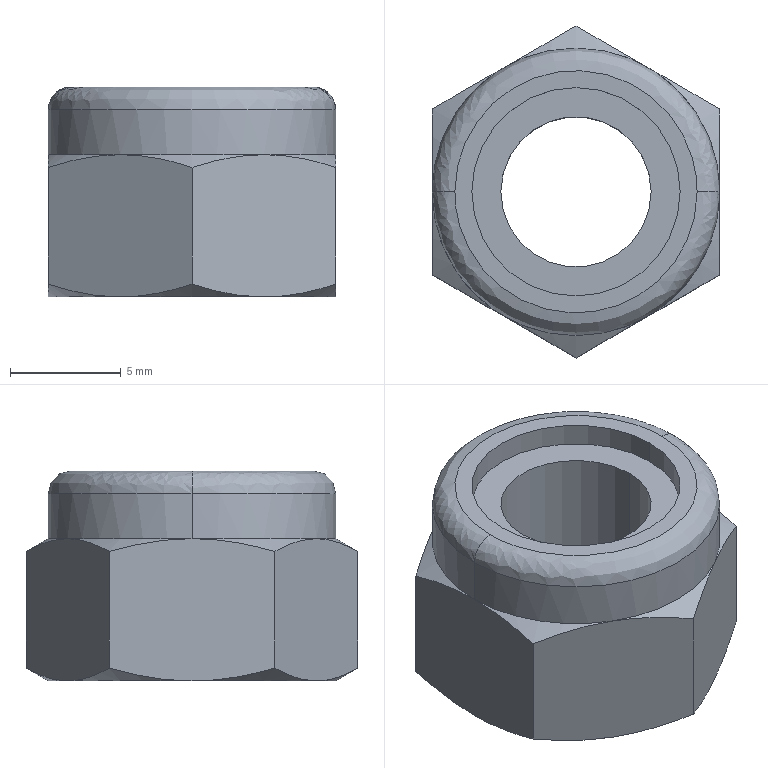Part | STEP file | Flat conveyor mechanism-prevailing torque nut style 1 insert_din_DIN EN ISO 7040 - M8 - N_Default | 1 solid | 33 faces | box 13 x 15.011 x 9.5 mm | volume 952.721 mm3 | cone 14 | plane 9 | cylinder 8 | spline 2 | commonest cylinder face diameters 6.8 x2 8 x2 9.429 x2 13 x2
STEP:
#1=CARTESIAN_POINT('',(5.48,0.,3.06));
#2=VERTEX_POINT('',#1);
#3=CARTESIAN_POINT('',(-5.48,0.,3.06));
#4=VERTEX_POINT('',#3);
#5=CARTESIAN_POINT('',(5.48,0.,3.06));
#6=CARTESIAN_POINT('',(5.48,-10.96,3.06));
#7=CARTESIAN_POINT('',(-5.48,-10.96,3.06));
#8=CARTESIAN_POINT('',(-5.48,0.,3.06));
#9=(BOUNDED_CURVE()B_SPLINE_CURVE(3,(#5,#6,#7,#8),.UNSPECIFIED.,.F.,.F.)B_SPLINE_CURVE_WITH_KNOTS((4,4),(0.,1.),.UNSPECIFIED.)CURVE()GEOMETRIC_REPRESENTATION_ITEM()RATIONAL_B_SPLINE_CURVE((1.,0.3333,0.3333,1.))REPRESENTATION_ITEM(''));
#10=EDGE_CURVE('',#2,#4,#9,.T.);
#11=ORIENTED_EDGE('',*,*,#10,.T.);
#12=CARTESIAN_POINT('',(-6.5,0.,2.04));
#13=VERTEX_POINT('',#12);
#14=CARTESIAN_POINT('',(-5.48,0.,2.04));
#15=DIRECTION('',(0.,-1.,0.));
#16=DIRECTION('',(-1.,0.,0.));
#17=AXIS2_PLACEMENT_3D('',#14,#15,#16);
#18=CIRCLE('',#17,1.02);
#19=EDGE_CURVE('',#4,#13,#18,.T.);
#20=ORIENTED_EDGE('',*,*,#19,.T.);
#21=CARTESIAN_POINT('',(6.5,0.,2.04));
#22=VERTEX_POINT('',#21);
#23=CARTESIAN_POINT('',(0.,0.,2.04));
#24=DIRECTION('',(0.,0.,1.));
#25=DIRECTION('',(1.,0.,0.));
#26=AXIS2_PLACEMENT_3D('',#23,#24,#25);
#27=CIRCLE('',#26,6.5);
#28=EDGE_CURVE('',#13,#22,#27,.T.);
#29=ORIENTED_EDGE('',*,*,#28,.T.);
#30=CARTESIAN_POINT('',(5.48,0.,2.04));
#31=DIRECTION('',(0.,1.,0.));
#32=DIRECTION('',(1.,0.,0.));
#33=AXIS2_PLACEMENT_3D('',#30,#31,#32);
#34=CIRCLE('',#33,1.02);
#35=EDGE_CURVE('',#2,#22,#34,.T.);
#36=ORIENTED_EDGE('',*,*,#35,.F.);
#37=EDGE_LOOP('',(#11,#20,#29,#36));
#38=FACE_OUTER_BOUND('',#37,.T.);
#39=CARTESIAN_POINT('',(-5.48,0.,3.06));
#40=CARTESIAN_POINT('',(-5.48,-10.96,3.06));
#41=CARTESIAN_POINT('',(5.48,-10.96,3.06));
#42=CARTESIAN_POINT('',(5.48,0.,3.06));
#43=CARTESIAN_POINT('',(-6.078,0.,3.06));
#44=CARTESIAN_POINT('',(-6.078,-12.155,3.06));
#45=CARTESIAN_POINT('',(6.078,-12.155,3.06));
#46=CARTESIAN_POINT('',(6.078,0.,3.06));
#47=CARTESIAN_POINT('',(-6.5,0.,2.638));
#48=CARTESIAN_POINT('',(-6.5,-13.,2.638));
#49=CARTESIAN_POINT('',(6.5,-13.,2.638));
#50=CARTESIAN_POINT('',(6.5,0.,2.638));
#51=CARTESIAN_POINT('',(-6.5,0.,2.04));
#52=CARTESIAN_POINT('',(-6.5,-13.,2.04));
#53=CARTESIAN_POINT('',(6.5,-13.,2.04));
#54=CARTESIAN_POINT('',(6.5,0.,2.04));
#55=(BOUNDED_SURFACE()B_SPLINE_SURFACE(3,3,((#39,#40,#41,#42),(#43,#44,#45,#46),(#47,#48,#49,#50),(#51,#52,#53,#54)),.UNSPECIFIED.,.F.,.F.,.T.)B_SPLINE_SURFACE_WITH_KNOTS((4,4),(4,4),(0.,1.),(0.,1.),.UNSPECIFIED.)GEOMETRIC_REPRESENTATION_ITEM()RATIONAL_B_SPLINE_SURFACE(((1.,0.3333,0.3333,1.),(0.8047,0.2682,0.2682,0.8047),(0.8047,0.2682,0.2682,0.8047),(1.,0.3333,0.3333,1.)))REPRESENTATION_ITEM('')SURFACE());
#56=ADVANCED_FACE('',(#38),#55,.T.);
#57=CARTESIAN_POINT('',(-3.4,0.,-5.994));
#58=VERTEX_POINT('',#57);
#59=CARTESIAN_POINT('',(3.4,0.,-5.994));
#60=VERTEX_POINT('',#59);
#61=CARTESIAN_POINT('',(0.,0.,-5.994));
#62=DIRECTION('',(0.,0.,1.));
#63=DIRECTION('',(1.,0.,0.));
#64=AXIS2_PLACEMENT_3D('',#61,#62,#63);
#65=CIRCLE('',#64,3.4);
#66=EDGE_CURVE('',#58,#60,#65,.T.);
#67=ORIENTED_EDGE('',*,*,#66,.F.);
#68=CARTESIAN_POINT('',(-3.4,0.,2.04));
#69=VERTEX_POINT('',#68);
#70=CARTESIAN_POINT('',(-3.4,0.,-6.44));
#71=DIRECTION('',(0.,0.,1.));
#72=VECTOR('',#71,1000.);
#73=LINE('',#70,#72);
#74=EDGE_CURVE('',#58,#69,#73,.T.);
#75=ORIENTED_EDGE('',*,*,#74,.T.);
#76=CARTESIAN_POINT('',(3.4,0.,2.04));
#77=VERTEX_POINT('',#76);
#78=CARTESIAN_POINT('',(0.,0.,2.04));
#79=DIRECTION('',(0.,0.,-1.));
#80=DIRECTION('',(1.,0.,0.));
#81=AXIS2_PLACEMENT_3D('',#78,#79,#80);
#82=CIRCLE('',#81,3.4);
#83=EDGE_CURVE('',#77,#69,#82,.T.);
#84=ORIENTED_EDGE('',*,*,#83,.F.);
#85=CARTESIAN_POINT('',(3.4,0.,-6.44));
#86=DIRECTION('',(0.,0.,1.));
#87=VECTOR('',#86,1000.);
#88=LINE('',#85,#87);
#89=EDGE_CURVE('',#60,#77,#88,.T.);
#90=ORIENTED_EDGE('',*,*,#89,.F.);
#91=EDGE_LOOP('',(#67,#75,#84,#90));
#92=FACE_OUTER_BOUND('',#91,.T.);
#93=CARTESIAN_POINT('',(0.,0.,-6.44));
#94=DIRECTION('',(0.,0.,1.));
#95=DIRECTION('',(1.,0.,0.));
#96=AXIS2_PLACEMENT_3D('',#93,#94,#95);
#97=CYLINDRICAL_SURFACE('',#96,3.4);
#98=ADVANCED_FACE('',(#92),#97,.F.);
#99=ORIENTED_EDGE('',*,*,#66,.T.);
#100=CARTESIAN_POINT('',(4.,0.,-6.415));
#101=VERTEX_POINT('',#100);
#102=CARTESIAN_POINT('',(4.,0.,-6.415));
#103=DIRECTION('',(0.8192,0.,-0.5736));
#104=VECTOR('',#103,1000.);
#105=LINE('',#102,#104);
#106=EDGE_CURVE('',#60,#101,#105,.T.);
#107=ORIENTED_EDGE('',*,*,#106,.T.);
#108=CARTESIAN_POINT('',(-4.,0.,-6.415));
#109=VERTEX_POINT('',#108);
#110=CARTESIAN_POINT('',(0.,0.,-6.415));
#111=DIRECTION('',(0.,0.,1.));
#112=DIRECTION('',(-1.,0.,0.));
#113=AXIS2_PLACEMENT_3D('',#110,#111,#112);
#114=CIRCLE('',#113,4.);
#115=EDGE_CURVE('',#109,#101,#114,.T.);
#116=ORIENTED_EDGE('',*,*,#115,.F.);
#117=CARTESIAN_POINT('',(-4.,0.,-6.415));
#118=DIRECTION('',(-0.8192,0.,-0.5736));
#119=VECTOR('',#118,1000.);
#120=LINE('',#117,#119);
#121=EDGE_CURVE('',#58,#109,#120,.T.);
#122=ORIENTED_EDGE('',*,*,#121,.F.);
#123=EDGE_LOOP('',(#99,#107,#116,#122));
#124=FACE_OUTER_BOUND('',#123,.T.);
#125=CARTESIAN_POINT('',(0.,0.,-6.415));
#126=DIRECTION('',(0.,0.,-1.));
#127=DIRECTION('',(-1.,0.,0.));
#128=AXIS2_PLACEMENT_3D('',#125,#126,#127);
#129=CONICAL_SURFACE('',#128,4.,0.9599);
#130=ADVANCED_FACE('',(#124),#129,.F.);
#131=CARTESIAN_POINT('',(-4.,0.,-6.44));
#132=VERTEX_POINT('',#131);
#133=CARTESIAN_POINT('',(4.,0.,-6.44));
#134=VERTEX_POINT('',#133);
#135=CARTESIAN_POINT('',(0.,0.,-6.44));
#136=DIRECTION('',(0.,0.,1.));
#137=DIRECTION('',(1.,0.,0.));
#138=AXIS2_PLACEMENT_3D('',#135,#136,#137);
#139=CIRCLE('',#138,4.);
#140=EDGE_CURVE('',#132,#134,#139,.T.);
#141=ORIENTED_EDGE('',*,*,#140,.F.);
#142=CARTESIAN_POINT('',(-4.,0.,-25.038));
#143=DIRECTION('',(0.,0.,1.));
#144=VECTOR('',#143,1000.);
#145=LINE('',#142,#144);
#146=EDGE_CURVE('',#132,#109,#145,.T.);
#147=ORIENTED_EDGE('',*,*,#146,.T.);
#148=ORIENTED_EDGE('',*,*,#115,.T.);
#149=CARTESIAN_POINT('',(4.,0.,-25.038));
#150=DIRECTION('',(0.,0.,1.));
#151=VECTOR('',#150,1000.);
#152=LINE('',#149,#151);
#153=EDGE_CURVE('',#134,#101,#152,.T.);
#154=ORIENTED_EDGE('',*,*,#153,.F.);
#155=EDGE_LOOP('',(#141,#147,#148,#154));
#156=FACE_OUTER_BOUND('',#155,.T.);
#157=CARTESIAN_POINT('',(0.,0.,-25.038));
#158=DIRECTION('',(0.,0.,1.));
#159=DIRECTION('',(1.,0.,0.));
#160=AXIS2_PLACEMENT_3D('',#157,#158,#159);
#161=CYLINDRICAL_SURFACE('',#160,4.);
#162=ADVANCED_FACE('',(#156),#161,.F.);
#163=CARTESIAN_POINT('',(4.714,0.,2.04));
#164=VERTEX_POINT('',#163);
#165=CARTESIAN_POINT('',(-4.714,0.,2.04));
#166=VERTEX_POINT('',#165);
#167=CARTESIAN_POINT('',(0.,0.,2.04));
#168=DIRECTION('',(0.,0.,-1.));
#169=DIRECTION('',(1.,0.,0.));
#170=AXIS2_PLACEMENT_3D('',#167,#168,#169);
#171=CIRCLE('',#170,4.714);
#172=EDGE_CURVE('',#164,#166,#171,.T.);
#173=ORIENTED_EDGE('',*,*,#172,.T.);
#174=CARTESIAN_POINT('',(-4.714,0.,3.06));
#175=VERTEX_POINT('',#174);
#176=CARTESIAN_POINT('',(-4.714,0.,9.481));
#177=DIRECTION('',(0.,0.,1.));
#178=VECTOR('',#177,1000.);
#179=LINE('',#176,#178);
#180=EDGE_CURVE('',#166,#175,#179,.T.);
#181=ORIENTED_EDGE('',*,*,#180,.T.);
#182=CARTESIAN_POINT('',(4.714,0.,3.06));
#183=VERTEX_POINT('',#182);
#184=CARTESIAN_POINT('',(0.,0.,3.06));
#185=DIRECTION('',(0.,0.,-1.));
#186=DIRECTION('',(1.,0.,0.));
#187=AXIS2_PLACEMENT_3D('',#184,#185,#186);
#188=CIRCLE('',#187,4.714);
#189=EDGE_CURVE('',#183,#175,#188,.T.);
#190=ORIENTED_EDGE('',*,*,#189,.F.);
#191=CARTESIAN_POINT('',(4.714,0.,9.481));
#192=DIRECTION('',(0.,0.,1.));
#193=VECTOR('',#192,1000.);
#194=LINE('',#191,#193);
#195=EDGE_CURVE('',#164,#183,#194,.T.);
#196=ORIENTED_EDGE('',*,*,#195,.F.);
#197=EDGE_LOOP('',(#173,#181,#190,#196));
#198=FACE_OUTER_BOUND('',#197,.T.);
#199=CARTESIAN_POINT('',(0.,0.,9.481));
#200=DIRECTION('',(0.,0.,1.));
#201=DIRECTION('',(1.,0.,0.));
#202=AXIS2_PLACEMENT_3D('',#199,#200,#201);
#203=CYLINDRICAL_SURFACE('',#202,4.714);
#204=ADVANCED_FACE('',(#198),#203,.F.);
#205=CARTESIAN_POINT('',(-3.25,5.629,0.));
#206=VERTEX_POINT('',#205);
#207=CARTESIAN_POINT('',(-6.5,0.,0.));
#208=VERTEX_POINT('',#207);
#209=CARTESIAN_POINT('',(0.,0.,0.));
#210=DIRECTION('',(0.,0.,1.));
#211=DIRECTION('',(1.,0.,0.));
#212=AXIS2_PLACEMENT_3D('',#209,#210,#211);
#213=CIRCLE('',#212,6.5);
#214=EDGE_CURVE('',#206,#208,#213,.T.);
#215=ORIENTED_EDGE('',*,*,#214,.T.);
#216=CARTESIAN_POINT('',(-6.5,0.,9.481));
#217=DIRECTION('',(0.,0.,1.));
#218=VECTOR('',#217,1000.);
#219=LINE('',#216,#218);
#220=EDGE_CURVE('',#208,#13,#219,.T.);
#221=ORIENTED_EDGE('',*,*,#220,.T.);
#222=CARTESIAN_POINT('',(0.,0.,2.04));
#223=DIRECTION('',(0.,0.,1.));
#224=DIRECTION('',(1.,0.,0.));
#225=AXIS2_PLACEMENT_3D('',#222,#223,#224);
#226=CIRCLE('',#225,6.5);
#227=EDGE_CURVE('',#22,#13,#226,.T.);
#228=ORIENTED_EDGE('',*,*,#227,.F.);
#229=CARTESIAN_POINT('',(6.5,0.,0.));
#230=VERTEX_POINT('',#229);
#231=CARTESIAN_POINT('',(6.5,0.,9.481));
#232=DIRECTION('',(0.,0.,1.));
#233=VECTOR('',#232,1000.);
#234=LINE('',#231,#233);
#235=EDGE_CURVE('',#230,#22,#234,.T.);
#236=ORIENTED_EDGE('',*,*,#235,.F.);
#237=CARTESIAN_POINT('',(3.25,5.629,0.));
#238=VERTEX_POINT('',#237);
#239=CARTESIAN_POINT('',(0.,0.,0.));
#240=DIRECTION('',(0.,0.,1.));
#241=DIRECTION('',(1.,0.,0.));
#242=AXIS2_PLACEMENT_3D('',#239,#240,#241);
#243=CIRCLE('',#242,6.5);
#244=EDGE_CURVE('',#230,#238,#243,.T.);
#245=ORIENTED_EDGE('',*,*,#244,.T.);
#246=CARTESIAN_POINT('',(0.,0.,0.));
#247=DIRECTION('',(0.,0.,1.));
#248=DIRECTION('',(1.,0.,0.));
#249=AXIS2_PLACEMENT_3D('',#246,#247,#248);
#250=CIRCLE('',#249,6.5);
#251=EDGE_CURVE('',#238,#206,#250,.T.);
#252=ORIENTED_EDGE('',*,*,#251,.T.);
#253=EDGE_LOOP('',(#215,#221,#228,#236,#245,#252));
#254=FACE_OUTER_BOUND('',#253,.T.);
#255=CARTESIAN_POINT('',(0.,0.,9.481));
#256=DIRECTION('',(0.,0.,1.));
#257=DIRECTION('',(1.,0.,0.));
#258=AXIS2_PLACEMENT_3D('',#255,#256,#257);
#259=CYLINDRICAL_SURFACE('',#258,6.5);
#260=ADVANCED_FACE('',(#254),#259,.T.);
#261=ORIENTED_EDGE('',*,*,#74,.F.);
#262=CARTESIAN_POINT('',(0.,0.,-5.994));
#263=DIRECTION('',(0.,0.,1.));
#264=DIRECTION('',(1.,0.,0.));
#265=AXIS2_PLACEMENT_3D('',#262,#263,#264);
#266=CIRCLE('',#265,3.4);
#267=EDGE_CURVE('',#60,#58,#266,.T.);
#268=ORIENTED_EDGE('',*,*,#267,.F.);
#269=ORIENTED_EDGE('',*,*,#89,.T.);
#270=CARTESIAN_POINT('',(0.,0.,2.04));
#271=DIRECTION('',(0.,0.,-1.));
#272=DIRECTION('',(1.,0.,0.));
#273=AXIS2_PLACEMENT_3D('',#270,#271,#272);
#274=CIRCLE('',#273,3.4);
#275=EDGE_CURVE('',#69,#77,#274,.T.);
#276=ORIENTED_EDGE('',*,*,#275,.F.);
#277=EDGE_LOOP('',(#261,#268,#269,#276));
#278=FACE_OUTER_BOUND('',#277,.T.);
#279=CARTESIAN_POINT('',(0.,0.,-6.44));
#280=DIRECTION('',(0.,0.,1.));
#281=DIRECTION('',(1.,0.,0.));
#282=AXIS2_PLACEMENT_3D('',#279,#280,#281);
#283=CYLINDRICAL_SURFACE('',#282,3.4);
#284=ADVANCED_FACE('',(#278),#283,.F.);
#285=ORIENTED_EDGE('',*,*,#106,.F.);
#286=ORIENTED_EDGE('',*,*,#267,.T.);
#287=ORIENTED_EDGE('',*,*,#121,.T.);
#288=CARTESIAN_POINT('',(0.,0.,-6.415));
#289=DIRECTION('',(0.,0.,1.));
#290=DIRECTION('',(-1.,0.,0.));
#291=AXIS2_PLACEMENT_3D('',#288,#289,#290);
#292=CIRCLE('',#291,4.);
#293=EDGE_CURVE('',#101,#109,#292,.T.);
#294=ORIENTED_EDGE('',*,*,#293,.F.);
#295=EDGE_LOOP('',(#285,#286,#287,#294));
#296=FACE_OUTER_BOUND('',#295,.T.);
#297=CARTESIAN_POINT('',(0.,0.,-6.415));
#298=DIRECTION('',(0.,0.,-1.));
#299=DIRECTION('',(-1.,0.,0.));
#300=AXIS2_PLACEMENT_3D('',#297,#298,#299);
#301=CONICAL_SURFACE('',#300,4.,0.9599);
#302=ADVANCED_FACE('',(#296),#301,.F.);
#303=ORIENTED_EDGE('',*,*,#172,.F.);
#304=CARTESIAN_POINT('',(0.,0.,2.04));
#305=DIRECTION('',(0.,0.,-1.));
#306=DIRECTION('',(1.,0.,0.));
#307=AXIS2_PLACEMENT_3D('',#304,#305,#306);
#308=CIRCLE('',#307,4.714);
#309=EDGE_CURVE('',#166,#164,#308,.T.);
#310=ORIENTED_EDGE('',*,*,#309,.F.);
#311=EDGE_LOOP('',(#303,#310));
#312=FACE_OUTER_BOUND('',#311,.T.);
#313=ORIENTED_EDGE('',*,*,#83,.T.);
#314=ORIENTED_EDGE('',*,*,#275,.T.);
#315=EDGE_LOOP('',(#313,#314));
#316=FACE_BOUND('',#315,.T.);
#317=CARTESIAN_POINT('',(0.,3.4,2.04));
#318=DIRECTION('',(0.,0.,-1.));
#319=DIRECTION('',(-1.,0.,0.));
#320=AXIS2_PLACEMENT_3D('',#317,#318,#319);
#321=PLANE('',#320);
#322=ADVANCED_FACE('',(#312,#316),#321,.F.);
#323=ORIENTED_EDGE('',*,*,#146,.F.);
#324=CARTESIAN_POINT('',(0.,0.,-6.44));
#325=DIRECTION('',(0.,0.,1.));
#326=DIRECTION('',(1.,0.,0.));
#327=AXIS2_PLACEMENT_3D('',#324,#325,#326);
#328=CIRCLE('',#327,4.);
#329=EDGE_CURVE('',#134,#132,#328,.T.);
#330=ORIENTED_EDGE('',*,*,#329,.F.);
#331=ORIENTED_EDGE('',*,*,#153,.T.);
#332=ORIENTED_EDGE('',*,*,#293,.T.);
#333=EDGE_LOOP('',(#323,#330,#331,#332));
#334=FACE_OUTER_BOUND('',#333,.T.);
#335=CARTESIAN_POINT('',(0.,0.,-25.038));
#336=DIRECTION('',(0.,0.,1.));
#337=DIRECTION('',(1.,0.,0.));
#338=AXIS2_PLACEMENT_3D('',#335,#336,#337);
#339=CYLINDRICAL_SURFACE('',#338,4.);
#340=ADVANCED_FACE('',(#334),#339,.F.);
#341=ORIENTED_EDGE('',*,*,#180,.F.);
#342=ORIENTED_EDGE('',*,*,#309,.T.);
#343=ORIENTED_EDGE('',*,*,#195,.T.);
#344=CARTESIAN_POINT('',(0.,0.,3.06));
#345=DIRECTION('',(0.,0.,-1.));
#346=DIRECTION('',(1.,0.,0.));
#347=AXIS2_PLACEMENT_3D('',#344,#345,#346);
#348=CIRCLE('',#347,4.714);
#349=EDGE_CURVE('',#175,#183,#348,.T.);
#350=ORIENTED_EDGE('',*,*,#349,.F.);
#351=EDGE_LOOP('',(#341,#342,#343,#350));
#352=FACE_OUTER_BOUND('',#351,.T.);
#353=CARTESIAN_POINT('',(0.,0.,9.481));
#354=DIRECTION('',(0.,0.,1.));
#355=DIRECTION('',(1.,0.,0.));
#356=AXIS2_PLACEMENT_3D('',#353,#354,#355);
#357=CYLINDRICAL_SURFACE('',#356,4.714);
#358=ADVANCED_FACE('',(#352),#357,.F.);
#359=CARTESIAN_POINT('',(3.25,-5.629,-6.44));
#360=VERTEX_POINT('',#359);
#361=CARTESIAN_POINT('',(6.5,0.,-6.44));
#362=VERTEX_POINT('',#361);
#363=CARTESIAN_POINT('',(0.,0.,-6.44));
#364=DIRECTION('',(0.,0.,1.));
#365=DIRECTION('',(1.,0.,0.));
#366=AXIS2_PLACEMENT_3D('',#363,#364,#365);
#367=CIRCLE('',#366,6.5);
#368=EDGE_CURVE('',#360,#362,#367,.T.);
#369=ORIENTED_EDGE('',*,*,#368,.F.);
#370=CARTESIAN_POINT('',(-3.25,-5.629,-6.44));
#371=VERTEX_POINT('',#370);
#372=CARTESIAN_POINT('',(0.,0.,-6.44));
#373=DIRECTION('',(0.,0.,1.));
#374=DIRECTION('',(1.,0.,0.));
#375=AXIS2_PLACEMENT_3D('',#372,#373,#374);
#376=CIRCLE('',#375,6.5);
#377=EDGE_CURVE('',#371,#360,#376,.T.);
#378=ORIENTED_EDGE('',*,*,#377,.F.);
#379=CARTESIAN_POINT('',(-6.5,0.,-6.44));
#380=VERTEX_POINT('',#379);
#381=CARTESIAN_POINT('',(0.,0.,-6.44));
#382=DIRECTION('',(0.,0.,1.));
#383=DIRECTION('',(1.,0.,0.));
#384=AXIS2_PLACEMENT_3D('',#381,#382,#383);
#385=CIRCLE('',#384,6.5);
#386=EDGE_CURVE('',#380,#371,#385,.T.);
#387=ORIENTED_EDGE('',*,*,#386,.F.);
#388=CARTESIAN_POINT('',(-3.25,5.629,-6.44));
#389=VERTEX_POINT('',#388);
#390=CARTESIAN_POINT('',(0.,0.,-6.44));
#391=DIRECTION('',(0.,0.,1.));
#392=DIRECTION('',(1.,0.,0.));
#393=AXIS2_PLACEMENT_3D('',#390,#391,#392);
#394=CIRCLE('',#393,6.5);
#395=EDGE_CURVE('',#389,#380,#394,.T.);
#396=ORIENTED_EDGE('',*,*,#395,.F.);
#397=CARTESIAN_POINT('',(3.25,5.629,-6.44));
#398=VERTEX_POINT('',#397);
#399=CARTESIAN_POINT('',(0.,0.,-6.44));
#400=DIRECTION('',(0.,0.,1.));
#401=DIRECTION('',(1.,0.,0.));
#402=AXIS2_PLACEMENT_3D('',#399,#400,#401);
#403=CIRCLE('',#402,6.5);
#404=EDGE_CURVE('',#398,#389,#403,.T.);
#405=ORIENTED_EDGE('',*,*,#404,.F.);
#406=CARTESIAN_POINT('',(0.,0.,-6.44));
#407=DIRECTION('',(0.,0.,1.));
#408=DIRECTION('',(1.,0.,0.));
#409=AXIS2_PLACEMENT_3D('',#406,#407,#408);
#410=CIRCLE('',#409,6.5);
#411=EDGE_CURVE('',#362,#398,#410,.T.);
#412=ORIENTED_EDGE('',*,*,#411,.F.);
#413=EDGE_LOOP('',(#369,#378,#387,#396,#405,#412));
#414=FACE_OUTER_BOUND('',#413,.T.);
#415=ORIENTED_EDGE('',*,*,#329,.T.);
#416=ORIENTED_EDGE('',*,*,#140,.T.);
#417=EDGE_LOOP('',(#415,#416));
#418=FACE_BOUND('',#417,.T.);
#419=CARTESIAN_POINT('',(-13.,0.,-6.44));
#420=DIRECTION('',(0.,0.,1.));
#421=DIRECTION('',(1.,0.,0.));
#422=AXIS2_PLACEMENT_3D('',#419,#420,#421);
#423=PLANE('',#422);
#424=ADVANCED_FACE('',(#414,#418),#423,.F.);
#425=ORIENTED_EDGE('',*,*,#10,.F.);
#426=CARTESIAN_POINT('',(-5.48,0.,3.06));
#427=CARTESIAN_POINT('',(-5.48,10.96,3.06));
#428=CARTESIAN_POINT('',(5.48,10.96,3.06));
#429=CARTESIAN_POINT('',(5.48,0.,3.06));
#430=(BOUNDED_CURVE()B_SPLINE_CURVE(3,(#426,#427,#428,#429),.UNSPECIFIED.,.F.,.T.)B_SPLINE_CURVE_WITH_KNOTS((4,4),(0.,1.),.UNSPECIFIED.)CURVE()GEOMETRIC_REPRESENTATION_ITEM()RATIONAL_B_SPLINE_CURVE((1.,0.3333,0.3333,1.))REPRESENTATION_ITEM(''));
#431=EDGE_CURVE('',#4,#2,#430,.T.);
#432=ORIENTED_EDGE('',*,*,#431,.F.);
#433=EDGE_LOOP('',(#425,#432));
#434=FACE_OUTER_BOUND('',#433,.T.);
#435=ORIENTED_EDGE('',*,*,#189,.T.);
#436=ORIENTED_EDGE('',*,*,#349,.T.);
#437=EDGE_LOOP('',(#435,#436));
#438=FACE_BOUND('',#437,.T.);
#439=CARTESIAN_POINT('',(0.,4.714,3.06));
#440=DIRECTION('',(0.,0.,-1.));
#441=DIRECTION('',(-1.,0.,0.));
#442=AXIS2_PLACEMENT_3D('',#439,#440,#441);
#443=PLANE('',#442);
#444=ADVANCED_FACE('',(#434,#438),#443,.F.);
#445=CARTESIAN_POINT('',(6.5,3.753,-5.859));
#446=VERTEX_POINT('',#445);
#447=CARTESIAN_POINT('',(6.5,3.753,-5.859));
#448=CARTESIAN_POINT('',(6.5,2.527,-6.213));
#449=CARTESIAN_POINT('',(6.5,1.281,-6.44));
#450=CARTESIAN_POINT('',(6.5,0.,-6.44));
#451=B_SPLINE_CURVE_WITH_KNOTS('',3,(#447,#448,#449,#450),.UNSPECIFIED.,.F.,.F.,(4,4),(0.,0.003797),.UNSPECIFIED.);
#452=EDGE_CURVE('',#446,#362,#451,.T.);
#453=ORIENTED_EDGE('',*,*,#452,.T.);
#454=ORIENTED_EDGE('',*,*,#411,.T.);
#455=CARTESIAN_POINT('',(3.25,5.629,-6.44));
#456=CARTESIAN_POINT('',(4.359,4.989,-6.44));
#457=CARTESIAN_POINT('',(5.438,4.366,-6.213));
#458=CARTESIAN_POINT('',(6.5,3.753,-5.859));
#459=B_SPLINE_CURVE_WITH_KNOTS('',3,(#455,#456,#457,#458),.UNSPECIFIED.,.F.,.F.,(4,4),(0.,0.003797),.UNSPECIFIED.);
#460=EDGE_CURVE('',#398,#446,#459,.T.);
#461=ORIENTED_EDGE('',*,*,#460,.T.);
#462=EDGE_LOOP('',(#453,#454,#461));
#463=FACE_OUTER_BOUND('',#462,.T.);
#464=CARTESIAN_POINT('',(0.,0.,-5.856));
#465=DIRECTION('',(0.,0.,1.));
#466=DIRECTION('',(1.,0.,0.));
#467=AXIS2_PLACEMENT_3D('',#464,#465,#466);
#468=CONICAL_SURFACE('',#467,7.512,1.047);
#469=ADVANCED_FACE('',(#463),#468,.T.);
#470=ORIENTED_EDGE('',*,*,#368,.T.);
#471=CARTESIAN_POINT('',(6.5,-3.753,-5.859));
#472=VERTEX_POINT('',#471);
#473=CARTESIAN_POINT('',(6.5,0.,-6.44));
#474=CARTESIAN_POINT('',(6.5,-1.281,-6.44));
#475=CARTESIAN_POINT('',(6.5,-2.527,-6.213));
#476=CARTESIAN_POINT('',(6.5,-3.753,-5.859));
#477=B_SPLINE_CURVE_WITH_KNOTS('',3,(#473,#474,#475,#476),.UNSPECIFIED.,.F.,.F.,(4,4),(0.,0.003797),.UNSPECIFIED.);
#478=EDGE_CURVE('',#362,#472,#477,.T.);
#479=ORIENTED_EDGE('',*,*,#478,.T.);
#480=CARTESIAN_POINT('',(6.5,-3.753,-5.859));
#481=CARTESIAN_POINT('',(5.438,-4.366,-6.213));
#482=CARTESIAN_POINT('',(4.359,-4.989,-6.44));
#483=CARTESIAN_POINT('',(3.25,-5.629,-6.44));
#484=B_SPLINE_CURVE_WITH_KNOTS('',3,(#480,#481,#482,#483),.UNSPECIFIED.,.F.,.F.,(4,4),(0.,0.003797),.UNSPECIFIED.);
#485=EDGE_CURVE('',#472,#360,#484,.T.);
#486=ORIENTED_EDGE('',*,*,#485,.T.);
#487=EDGE_LOOP('',(#470,#479,#486));
#488=FACE_OUTER_BOUND('',#487,.T.);
#489=CARTESIAN_POINT('',(0.,0.,-5.856));
#490=DIRECTION('',(0.,0.,1.));
#491=DIRECTION('',(1.,0.,0.));
#492=AXIS2_PLACEMENT_3D('',#489,#490,#491);
#493=CONICAL_SURFACE('',#492,7.512,1.047);
#494=ADVANCED_FACE('',(#488),#493,.T.);
#495=CARTESIAN_POINT('',(0.000000038,-7.506,-5.859));
#496=VERTEX_POINT('',#495);
#497=CARTESIAN_POINT('',(0.000000038,-7.506,-5.859));
#498=CARTESIAN_POINT('',(-1.062,-6.892,-6.213));
#499=CARTESIAN_POINT('',(-2.141,-6.27,-6.44));
#500=CARTESIAN_POINT('',(-3.25,-5.629,-6.44));
#501=B_SPLINE_CURVE_WITH_KNOTS('',3,(#497,#498,#499,#500),.UNSPECIFIED.,.F.,.F.,(4,4),(0.,0.003797),.UNSPECIFIED.);
#502=EDGE_CURVE('',#496,#371,#501,.T.);
#503=ORIENTED_EDGE('',*,*,#502,.T.);
#504=ORIENTED_EDGE('',*,*,#377,.T.);
#505=CARTESIAN_POINT('',(3.25,-5.629,-6.44));
#506=CARTESIAN_POINT('',(2.141,-6.27,-6.44));
#507=CARTESIAN_POINT('',(1.062,-6.892,-6.213));
#508=CARTESIAN_POINT('',(0.000000038,-7.506,-5.859));
#509=B_SPLINE_CURVE_WITH_KNOTS('',3,(#505,#506,#507,#508),.UNSPECIFIED.,.F.,.F.,(4,4),(0.,0.003797),.UNSPECIFIED.);
#510=EDGE_CURVE('',#360,#496,#509,.T.);
#511=ORIENTED_EDGE('',*,*,#510,.T.);
#512=EDGE_LOOP('',(#503,#504,#511));
#513=FACE_OUTER_BOUND('',#512,.T.);
#514=CARTESIAN_POINT('',(0.,0.,-5.856));
#515=DIRECTION('',(0.,0.,1.));
#516=DIRECTION('',(1.,0.,0.));
#517=AXIS2_PLACEMENT_3D('',#514,#515,#516);
#518=CONICAL_SURFACE('',#517,7.512,1.047);
#519=ADVANCED_FACE('',(#513),#518,.T.);
#520=CARTESIAN_POINT('',(-6.5,-3.753,-5.859));
#521=VERTEX_POINT('',#520);
#522=CARTESIAN_POINT('',(-6.5,-3.753,-5.859));
#523=CARTESIAN_POINT('',(-6.5,-2.527,-6.213));
#524=CARTESIAN_POINT('',(-6.5,-1.281,-6.44));
#525=CARTESIAN_POINT('',(-6.5,0.,-6.44));
#526=B_SPLINE_CURVE_WITH_KNOTS('',3,(#522,#523,#524,#525),.UNSPECIFIED.,.F.,.F.,(4,4),(0.,0.003797),.UNSPECIFIED.);
#527=EDGE_CURVE('',#521,#380,#526,.T.);
#528=ORIENTED_EDGE('',*,*,#527,.T.);
#529=ORIENTED_EDGE('',*,*,#386,.T.);
#530=CARTESIAN_POINT('',(-3.25,-5.629,-6.44));
#531=CARTESIAN_POINT('',(-4.359,-4.989,-6.44));
#532=CARTESIAN_POINT('',(-5.438,-4.366,-6.213));
#533=CARTESIAN_POINT('',(-6.5,-3.753,-5.859));
#534=B_SPLINE_CURVE_WITH_KNOTS('',3,(#530,#531,#532,#533),.UNSPECIFIED.,.F.,.F.,(4,4),(0.,0.003797),.UNSPECIFIED.);
#535=EDGE_CURVE('',#371,#521,#534,.T.);
#536=ORIENTED_EDGE('',*,*,#535,.T.);
#537=EDGE_LOOP('',(#528,#529,#536));
#538=FACE_OUTER_BOUND('',#537,.T.);
#539=CARTESIAN_POINT('',(0.,0.,-5.856));
#540=DIRECTION('',(0.,0.,1.));
#541=DIRECTION('',(1.,0.,0.));
#542=AXIS2_PLACEMENT_3D('',#539,#540,#541);
#543=CONICAL_SURFACE('',#542,7.512,1.047);
#544=ADVANCED_FACE('',(#538),#543,.T.);
#545=ORIENTED_EDGE('',*,*,#395,.T.);
#546=CARTESIAN_POINT('',(-6.5,3.753,-5.859));
#547=VERTEX_POINT('',#546);
#548=CARTESIAN_POINT('',(-6.5,0.,-6.44));
#549=CARTESIAN_POINT('',(-6.5,1.281,-6.44));
#550=CARTESIAN_POINT('',(-6.5,2.527,-6.213));
#551=CARTESIAN_POINT('',(-6.5,3.753,-5.859));
#552=B_SPLINE_CURVE_WITH_KNOTS('',3,(#548,#549,#550,#551),.UNSPECIFIED.,.F.,.F.,(4,4),(0.,0.003797),.UNSPECIFIED.);
#553=EDGE_CURVE('',#380,#547,#552,.T.);
#554=ORIENTED_EDGE('',*,*,#553,.T.);
#555=CARTESIAN_POINT('',(-6.5,3.753,-5.859));
#556=CARTESIAN_POINT('',(-5.438,4.366,-6.213));
#557=CARTESIAN_POINT('',(-4.359,4.989,-6.44));
#558=CARTESIAN_POINT('',(-3.25,5.629,-6.44));
#559=B_SPLINE_CURVE_WITH_KNOTS('',3,(#555,#556,#557,#558),.UNSPECIFIED.,.F.,.F.,(4,4),(0.,0.003797),.UNSPECIFIED.);
#560=EDGE_CURVE('',#547,#389,#559,.T.);
#561=ORIENTED_EDGE('',*,*,#560,.T.);
#562=EDGE_LOOP('',(#545,#554,#561));
#563=FACE_OUTER_BOUND('',#562,.T.);
#564=CARTESIAN_POINT('',(0.,0.,-5.856));
#565=DIRECTION('',(0.,0.,1.));
#566=DIRECTION('',(1.,0.,0.));
#567=AXIS2_PLACEMENT_3D('',#564,#565,#566);
#568=CONICAL_SURFACE('',#567,7.512,1.047);
#569=ADVANCED_FACE('',(#563),#568,.T.);
#570=CARTESIAN_POINT('',(-0.000000038,7.506,-5.859));
#571=VERTEX_POINT('',#570);
#572=CARTESIAN_POINT('',(-0.000000038,7.506,-5.859));
#573=CARTESIAN_POINT('',(1.062,6.892,-6.213));
#574=CARTESIAN_POINT('',(2.141,6.27,-6.44));
#575=CARTESIAN_POINT('',(3.25,5.629,-6.44));
#576=B_SPLINE_CURVE_WITH_KNOTS('',3,(#572,#573,#574,#575),.UNSPECIFIED.,.F.,.F.,(4,4),(0.,0.003797),.UNSPECIFIED.);
#577=EDGE_CURVE('',#571,#398,#576,.T.);
#578=ORIENTED_EDGE('',*,*,#577,.T.);
#579=ORIENTED_EDGE('',*,*,#404,.T.);
#580=CARTESIAN_POINT('',(-3.25,5.629,-6.44));
#581=CARTESIAN_POINT('',(-2.141,6.27,-6.44));
#582=CARTESIAN_POINT('',(-1.062,6.892,-6.213));
#583=CARTESIAN_POINT('',(-0.000000038,7.506,-5.859));
#584=B_SPLINE_CURVE_WITH_KNOTS('',3,(#580,#581,#582,#583),.UNSPECIFIED.,.F.,.F.,(4,4),(0.,0.003797),.UNSPECIFIED.);
#585=EDGE_CURVE('',#389,#571,#584,.T.);
#586=ORIENTED_EDGE('',*,*,#585,.T.);
#587=EDGE_LOOP('',(#578,#579,#586));
#588=FACE_OUTER_BOUND('',#587,.T.);
#589=CARTESIAN_POINT('',(0.,0.,-5.856));
#590=DIRECTION('',(0.,0.,1.));
#591=DIRECTION('',(1.,0.,0.));
#592=AXIS2_PLACEMENT_3D('',#589,#590,#591);
#593=CONICAL_SURFACE('',#592,7.512,1.047);
#594=ADVANCED_FACE('',(#588),#593,.T.);
#595=ORIENTED_EDGE('',*,*,#19,.F.);
#596=ORIENTED_EDGE('',*,*,#431,.T.);
#597=ORIENTED_EDGE('',*,*,#35,.T.);
#598=ORIENTED_EDGE('',*,*,#227,.T.);
#599=EDGE_LOOP('',(#595,#596,#597,#598));
#600=FACE_OUTER_BOUND('',#599,.T.);
#601=CARTESIAN_POINT('',(5.48,0.,3.06));
#602=CARTESIAN_POINT('',(5.48,10.96,3.06));
#603=CARTESIAN_POINT('',(-5.48,10.96,3.06));
#604=CARTESIAN_POINT('',(-5.48,0.,3.06));
#605=CARTESIAN_POINT('',(6.078,0.,3.06));
#606=CARTESIAN_POINT('',(6.078,12.155,3.06));
#607=CARTESIAN_POINT('',(-6.078,12.155,3.06));
#608=CARTESIAN_POINT('',(-6.078,0.,3.06));
#609=CARTESIAN_POINT('',(6.5,0.,2.638));
#610=CARTESIAN_POINT('',(6.5,13.,2.638));
#611=CARTESIAN_POINT('',(-6.5,13.,2.638));
#612=CARTESIAN_POINT('',(-6.5,0.,2.638));
#613=CARTESIAN_POINT('',(6.5,0.,2.04));
#614=CARTESIAN_POINT('',(6.5,13.,2.04));
#615=CARTESIAN_POINT('',(-6.5,13.,2.04));
#616=CARTESIAN_POINT('',(-6.5,0.,2.04));
#617=(BOUNDED_SURFACE()B_SPLINE_SURFACE(3,3,((#601,#602,#603,#604),(#605,#606,#607,#608),(#609,#610,#611,#612),(#613,#614,#615,#616)),.UNSPECIFIED.,.F.,.F.,.T.)B_SPLINE_SURFACE_WITH_KNOTS((4,4),(4,4),(0.,1.),(0.,1.),.UNSPECIFIED.)GEOMETRIC_REPRESENTATION_ITEM()RATIONAL_B_SPLINE_SURFACE(((1.,0.3333,0.3333,1.),(0.8047,0.2682,0.2682,0.8047),(0.8047,0.2682,0.2682,0.8047),(1.,0.3333,0.3333,1.)))REPRESENTATION_ITEM('')SURFACE());
#618=ADVANCED_FACE('',(#600),#617,.T.);
#619=CARTESIAN_POINT('',(6.5,-3.753,-0.5806));
#620=VERTEX_POINT('',#619);
#621=CARTESIAN_POINT('',(6.5,-3.753,-6.44));
#622=DIRECTION('',(0.,0.,1.));
#623=VECTOR('',#622,1000.);
#624=LINE('',#621,#623);
#625=EDGE_CURVE('',#472,#620,#624,.T.);
#626=ORIENTED_EDGE('',*,*,#625,.F.);
#627=ORIENTED_EDGE('',*,*,#478,.F.);
#628=ORIENTED_EDGE('',*,*,#452,.F.);
#629=CARTESIAN_POINT('',(6.5,3.753,-0.5806));
#630=VERTEX_POINT('',#629);
#631=CARTESIAN_POINT('',(6.5,3.753,-6.44));
#632=DIRECTION('',(0.,0.,-1.));
#633=VECTOR('',#632,1000.);
#634=LINE('',#631,#633);
#635=EDGE_CURVE('',#630,#446,#634,.T.);
#636=ORIENTED_EDGE('',*,*,#635,.F.);
#637=CARTESIAN_POINT('',(6.5,0.,0.));
#638=CARTESIAN_POINT('',(6.5,1.281,0.));
#639=CARTESIAN_POINT('',(6.5,2.527,-0.2266));
#640=CARTESIAN_POINT('',(6.5,3.753,-0.5806));
#641=B_SPLINE_CURVE_WITH_KNOTS('',3,(#637,#638,#639,#640),.UNSPECIFIED.,.F.,.F.,(4,4),(0.,0.003797),.UNSPECIFIED.);
#642=EDGE_CURVE('',#230,#630,#641,.T.);
#643=ORIENTED_EDGE('',*,*,#642,.F.);
#644=CARTESIAN_POINT('',(6.5,-3.753,-0.5806));
#645=CARTESIAN_POINT('',(6.5,-2.527,-0.2266));
#646=CARTESIAN_POINT('',(6.5,-1.281,0.));
#647=CARTESIAN_POINT('',(6.5,0.,0.));
#648=B_SPLINE_CURVE_WITH_KNOTS('',3,(#644,#645,#646,#647),.UNSPECIFIED.,.F.,.F.,(4,4),(0.,0.003797),.UNSPECIFIED.);
#649=EDGE_CURVE('',#620,#230,#648,.T.);
#650=ORIENTED_EDGE('',*,*,#649,.F.);
#651=EDGE_LOOP('',(#626,#627,#628,#636,#643,#650));
#652=FACE_OUTER_BOUND('',#651,.T.);
#653=CARTESIAN_POINT('',(6.5,3.753,-6.44));
#654=DIRECTION('',(-1.,0.,0.));
#655=DIRECTION('',(0.,0.,1.));
#656=AXIS2_PLACEMENT_3D('',#653,#654,#655);
#657=PLANE('',#656);
#658=ADVANCED_FACE('',(#652),#657,.F.);
#659=ORIENTED_EDGE('',*,*,#460,.F.);
#660=ORIENTED_EDGE('',*,*,#577,.F.);
#661=CARTESIAN_POINT('',(0.,7.506,-0.5806));
#662=VERTEX_POINT('',#661);
#663=CARTESIAN_POINT('',(0.,7.506,-6.44));
#664=DIRECTION('',(0.,0.,1.));
#665=VECTOR('',#664,1000.);
#666=LINE('',#663,#665);
#667=EDGE_CURVE('',#571,#662,#666,.T.);
#668=ORIENTED_EDGE('',*,*,#667,.T.);
#669=CARTESIAN_POINT('',(0.,7.506,-0.5806));
#670=CARTESIAN_POINT('',(1.062,6.892,-0.2266));
#671=CARTESIAN_POINT('',(2.141,6.27,0.));
#672=CARTESIAN_POINT('',(3.25,5.629,0.));
#673=B_SPLINE_CURVE_WITH_KNOTS('',3,(#669,#670,#671,#672),.UNSPECIFIED.,.F.,.F.,(4,4),(0.,0.003797),.UNSPECIFIED.);
#674=EDGE_CURVE('',#662,#238,#673,.T.);
#675=ORIENTED_EDGE('',*,*,#674,.T.);
#676=CARTESIAN_POINT('',(3.25,5.629,0.));
#677=CARTESIAN_POINT('',(4.359,4.989,0.));
#678=CARTESIAN_POINT('',(5.438,4.366,-0.2266));
#679=CARTESIAN_POINT('',(6.5,3.753,-0.5806));
#680=B_SPLINE_CURVE_WITH_KNOTS('',3,(#676,#677,#678,#679),.UNSPECIFIED.,.F.,.F.,(4,4),(0.,0.003797),.UNSPECIFIED.);
#681=EDGE_CURVE('',#238,#630,#680,.T.);
#682=ORIENTED_EDGE('',*,*,#681,.T.);
#683=ORIENTED_EDGE('',*,*,#635,.T.);
#684=EDGE_LOOP('',(#659,#660,#668,#675,#682,#683));
#685=FACE_OUTER_BOUND('',#684,.T.);
#686=CARTESIAN_POINT('',(6.5,3.753,-6.44));
#687=DIRECTION('',(0.5,0.866,0.));
#688=DIRECTION('',(-0.866,0.5,0.));
#689=AXIS2_PLACEMENT_3D('',#686,#687,#688);
#690=PLANE('',#689);
#691=ADVANCED_FACE('',(#685),#690,.T.);
#692=ORIENTED_EDGE('',*,*,#510,.F.);
#693=ORIENTED_EDGE('',*,*,#485,.F.);
#694=ORIENTED_EDGE('',*,*,#625,.T.);
#695=CARTESIAN_POINT('',(3.25,-5.629,0.));
#696=VERTEX_POINT('',#695);
#697=CARTESIAN_POINT('',(6.5,-3.753,-0.5806));
#698=CARTESIAN_POINT('',(5.438,-4.366,-0.2266));
#699=CARTESIAN_POINT('',(4.359,-4.989,0.));
#700=CARTESIAN_POINT('',(3.25,-5.629,0.));
#701=B_SPLINE_CURVE_WITH_KNOTS('',3,(#697,#698,#699,#700),.UNSPECIFIED.,.F.,.F.,(4,4),(0.,0.003797),.UNSPECIFIED.);
#702=EDGE_CURVE('',#620,#696,#701,.T.);
#703=ORIENTED_EDGE('',*,*,#702,.T.);
#704=CARTESIAN_POINT('',(0.,-7.506,-0.5806));
#705=VERTEX_POINT('',#704);
#706=CARTESIAN_POINT('',(3.25,-5.629,0.));
#707=CARTESIAN_POINT('',(2.141,-6.27,0.));
#708=CARTESIAN_POINT('',(1.062,-6.892,-0.2266));
#709=CARTESIAN_POINT('',(0.,-7.506,-0.5806));
#710=B_SPLINE_CURVE_WITH_KNOTS('',3,(#706,#707,#708,#709),.UNSPECIFIED.,.F.,.F.,(4,4),(0.,0.003797),.UNSPECIFIED.);
#711=EDGE_CURVE('',#696,#705,#710,.T.);
#712=ORIENTED_EDGE('',*,*,#711,.T.);
#713=CARTESIAN_POINT('',(0.,-7.506,-6.44));
#714=DIRECTION('',(0.,0.,-1.));
#715=VECTOR('',#714,1000.);
#716=LINE('',#713,#715);
#717=EDGE_CURVE('',#705,#496,#716,.T.);
#718=ORIENTED_EDGE('',*,*,#717,.T.);
#719=EDGE_LOOP('',(#692,#693,#694,#703,#712,#718));
#720=FACE_OUTER_BOUND('',#719,.T.);
#721=CARTESIAN_POINT('',(0.,-7.506,-6.44));
#722=DIRECTION('',(0.5,-0.866,0.));
#723=DIRECTION('',(0.866,0.5,0.));
#724=AXIS2_PLACEMENT_3D('',#721,#722,#723);
#725=PLANE('',#724);
#726=ADVANCED_FACE('',(#720),#725,.T.);
#727=ORIENTED_EDGE('',*,*,#535,.F.);
#728=ORIENTED_EDGE('',*,*,#502,.F.);
#729=ORIENTED_EDGE('',*,*,#717,.F.);
#730=CARTESIAN_POINT('',(-3.25,-5.629,0.));
#731=VERTEX_POINT('',#730);
#732=CARTESIAN_POINT('',(0.,-7.506,-0.5806));
#733=CARTESIAN_POINT('',(-1.062,-6.892,-0.2266));
#734=CARTESIAN_POINT('',(-2.141,-6.27,0.));
#735=CARTESIAN_POINT('',(-3.25,-5.629,0.));
#736=B_SPLINE_CURVE_WITH_KNOTS('',3,(#732,#733,#734,#735),.UNSPECIFIED.,.F.,.F.,(4,4),(0.,0.003797),.UNSPECIFIED.);
#737=EDGE_CURVE('',#705,#731,#736,.T.);
#738=ORIENTED_EDGE('',*,*,#737,.T.);
#739=CARTESIAN_POINT('',(-6.5,-3.753,-0.5806));
#740=VERTEX_POINT('',#739);
#741=CARTESIAN_POINT('',(-3.25,-5.629,0.));
#742=CARTESIAN_POINT('',(-4.359,-4.989,0.));
#743=CARTESIAN_POINT('',(-5.438,-4.366,-0.2266));
#744=CARTESIAN_POINT('',(-6.5,-3.753,-0.5806));
#745=B_SPLINE_CURVE_WITH_KNOTS('',3,(#741,#742,#743,#744),.UNSPECIFIED.,.F.,.F.,(4,4),(0.,0.003797),.UNSPECIFIED.);
#746=EDGE_CURVE('',#731,#740,#745,.T.);
#747=ORIENTED_EDGE('',*,*,#746,.T.);
#748=CARTESIAN_POINT('',(-6.5,-3.753,-6.44));
#749=DIRECTION('',(0.,0.,-1.));
#750=VECTOR('',#749,1000.);
#751=LINE('',#748,#750);
#752=EDGE_CURVE('',#740,#521,#751,.T.);
#753=ORIENTED_EDGE('',*,*,#752,.T.);
#754=EDGE_LOOP('',(#727,#728,#729,#738,#747,#753));
#755=FACE_OUTER_BOUND('',#754,.T.);
#756=CARTESIAN_POINT('',(-6.5,-3.753,-6.44));
#757=DIRECTION('',(-0.5,-0.866,0.));
#758=DIRECTION('',(0.866,-0.5,0.));
#759=AXIS2_PLACEMENT_3D('',#756,#757,#758);
#760=PLANE('',#759);
#761=ADVANCED_FACE('',(#755),#760,.T.);
#762=ORIENTED_EDGE('',*,*,#553,.F.);
#763=ORIENTED_EDGE('',*,*,#527,.F.);
#764=ORIENTED_EDGE('',*,*,#752,.F.);
#765=CARTESIAN_POINT('',(-6.5,-3.753,-0.5806));
#766=CARTESIAN_POINT('',(-6.5,-2.527,-0.2266));
#767=CARTESIAN_POINT('',(-6.5,-1.281,0.));
#768=CARTESIAN_POINT('',(-6.5,0.,0.));
#769=B_SPLINE_CURVE_WITH_KNOTS('',3,(#765,#766,#767,#768),.UNSPECIFIED.,.F.,.F.,(4,4),(0.,0.003797),.UNSPECIFIED.);
#770=EDGE_CURVE('',#740,#208,#769,.T.);
#771=ORIENTED_EDGE('',*,*,#770,.T.);
#772=CARTESIAN_POINT('',(-6.5,3.753,-0.5806));
#773=VERTEX_POINT('',#772);
#774=CARTESIAN_POINT('',(-6.5,0.,0.));
#775=CARTESIAN_POINT('',(-6.5,1.281,0.));
#776=CARTESIAN_POINT('',(-6.5,2.527,-0.2266));
#777=CARTESIAN_POINT('',(-6.5,3.753,-0.5806));
#778=B_SPLINE_CURVE_WITH_KNOTS('',3,(#774,#775,#776,#777),.UNSPECIFIED.,.F.,.F.,(4,4),(0.,0.003797),.UNSPECIFIED.);
#779=EDGE_CURVE('',#208,#773,#778,.T.);
#780=ORIENTED_EDGE('',*,*,#779,.T.);
#781=CARTESIAN_POINT('',(-6.5,3.753,-6.44));
#782=DIRECTION('',(0.,0.,-1.));
#783=VECTOR('',#782,1000.);
#784=LINE('',#781,#783);
#785=EDGE_CURVE('',#773,#547,#784,.T.);
#786=ORIENTED_EDGE('',*,*,#785,.T.);
#787=EDGE_LOOP('',(#762,#763,#764,#771,#780,#786));
#788=FACE_OUTER_BOUND('',#787,.T.);
#789=CARTESIAN_POINT('',(-6.5,3.753,-6.44));
#790=DIRECTION('',(-1.,0.,0.));
#791=DIRECTION('',(0.,0.,1.));
#792=AXIS2_PLACEMENT_3D('',#789,#790,#791);
#793=PLANE('',#792);
#794=ADVANCED_FACE('',(#788),#793,.T.);
#795=ORIENTED_EDGE('',*,*,#585,.F.);
#796=ORIENTED_EDGE('',*,*,#560,.F.);
#797=ORIENTED_EDGE('',*,*,#785,.F.);
#798=CARTESIAN_POINT('',(-6.5,3.753,-0.5806));
#799=CARTESIAN_POINT('',(-5.438,4.366,-0.2266));
#800=CARTESIAN_POINT('',(-4.359,4.989,0.));
#801=CARTESIAN_POINT('',(-3.25,5.629,0.));
#802=B_SPLINE_CURVE_WITH_KNOTS('',3,(#798,#799,#800,#801),.UNSPECIFIED.,.F.,.F.,(4,4),(0.,0.003797),.UNSPECIFIED.);
#803=EDGE_CURVE('',#773,#206,#802,.T.);
#804=ORIENTED_EDGE('',*,*,#803,.T.);
#805=CARTESIAN_POINT('',(-3.25,5.629,0.));
#806=CARTESIAN_POINT('',(-2.141,6.27,0.));
#807=CARTESIAN_POINT('',(-1.062,6.892,-0.2266));
#808=CARTESIAN_POINT('',(0.,7.506,-0.5806));
#809=B_SPLINE_CURVE_WITH_KNOTS('',3,(#805,#806,#807,#808),.UNSPECIFIED.,.F.,.F.,(4,4),(0.,0.003797),.UNSPECIFIED.);
#810=EDGE_CURVE('',#206,#662,#809,.T.);
#811=ORIENTED_EDGE('',*,*,#810,.T.);
#812=ORIENTED_EDGE('',*,*,#667,.F.);
#813=EDGE_LOOP('',(#795,#796,#797,#804,#811,#812));
#814=FACE_OUTER_BOUND('',#813,.T.);
#815=CARTESIAN_POINT('',(0.,7.506,-6.44));
#816=DIRECTION('',(-0.5,0.866,0.));
#817=DIRECTION('',(-0.866,-0.5,0.));
#818=AXIS2_PLACEMENT_3D('',#815,#816,#817);
#819=PLANE('',#818);
#820=ADVANCED_FACE('',(#814),#819,.T.);
#821=ORIENTED_EDGE('',*,*,#220,.F.);
#822=CARTESIAN_POINT('',(0.,0.,0.));
#823=DIRECTION('',(0.,0.,1.));
#824=DIRECTION('',(1.,0.,0.));
#825=AXIS2_PLACEMENT_3D('',#822,#823,#824);
#826=CIRCLE('',#825,6.5);
#827=EDGE_CURVE('',#208,#731,#826,.T.);
#828=ORIENTED_EDGE('',*,*,#827,.T.);
#829=CARTESIAN_POINT('',(0.,0.,0.));
#830=DIRECTION('',(0.,0.,1.));
#831=DIRECTION('',(1.,0.,0.));
#832=AXIS2_PLACEMENT_3D('',#829,#830,#831);
#833=CIRCLE('',#832,6.5);
#834=EDGE_CURVE('',#731,#696,#833,.T.);
#835=ORIENTED_EDGE('',*,*,#834,.T.);
#836=CARTESIAN_POINT('',(0.,0.,0.));
#837=DIRECTION('',(0.,0.,1.));
#838=DIRECTION('',(1.,0.,0.));
#839=AXIS2_PLACEMENT_3D('',#836,#837,#838);
#840=CIRCLE('',#839,6.5);
#841=EDGE_CURVE('',#696,#230,#840,.T.);
#842=ORIENTED_EDGE('',*,*,#841,.T.);
#843=ORIENTED_EDGE('',*,*,#235,.T.);
#844=ORIENTED_EDGE('',*,*,#28,.F.);
#845=EDGE_LOOP('',(#821,#828,#835,#842,#843,#844));
#846=FACE_OUTER_BOUND('',#845,.T.);
#847=CARTESIAN_POINT('',(0.,0.,9.481));
#848=DIRECTION('',(0.,0.,1.));
#849=DIRECTION('',(1.,0.,0.));
#850=AXIS2_PLACEMENT_3D('',#847,#848,#849);
#851=CYLINDRICAL_SURFACE('',#850,6.5);
#852=ADVANCED_FACE('',(#846),#851,.T.);
#853=ORIENTED_EDGE('',*,*,#841,.F.);
#854=ORIENTED_EDGE('',*,*,#702,.F.);
#855=ORIENTED_EDGE('',*,*,#649,.T.);
#856=EDGE_LOOP('',(#853,#854,#855));
#857=FACE_OUTER_BOUND('',#856,.T.);
#858=CARTESIAN_POINT('',(0.,0.,-0.584));
#859=DIRECTION('',(0.,0.,-1.));
#860=DIRECTION('',(-1.,0.,0.));
#861=AXIS2_PLACEMENT_3D('',#858,#859,#860);
#862=CONICAL_SURFACE('',#861,7.512,1.047);
#863=ADVANCED_FACE('',(#857),#862,.T.);
#864=ORIENTED_EDGE('',*,*,#642,.T.);
#865=ORIENTED_EDGE('',*,*,#681,.F.);
#866=ORIENTED_EDGE('',*,*,#244,.F.);
#867=EDGE_LOOP('',(#864,#865,#866));
#868=FACE_OUTER_BOUND('',#867,.T.);
#869=CARTESIAN_POINT('',(0.,0.,-0.584));
#870=DIRECTION('',(0.,0.,-1.));
#871=DIRECTION('',(-1.,0.,0.));
#872=AXIS2_PLACEMENT_3D('',#869,#870,#871);
#873=CONICAL_SURFACE('',#872,7.512,1.047);
#874=ADVANCED_FACE('',(#868),#873,.T.);
#875=ORIENTED_EDGE('',*,*,#674,.F.);
#876=ORIENTED_EDGE('',*,*,#810,.F.);
#877=ORIENTED_EDGE('',*,*,#251,.F.);
#878=EDGE_LOOP('',(#875,#876,#877));
#879=FACE_OUTER_BOUND('',#878,.T.);
#880=CARTESIAN_POINT('',(0.,0.,-0.584));
#881=DIRECTION('',(0.,0.,-1.));
#882=DIRECTION('',(-1.,0.,0.));
#883=AXIS2_PLACEMENT_3D('',#880,#881,#882);
#884=CONICAL_SURFACE('',#883,7.512,1.047);
#885=ADVANCED_FACE('',(#879),#884,.T.);
#886=ORIENTED_EDGE('',*,*,#737,.F.);
#887=ORIENTED_EDGE('',*,*,#711,.F.);
#888=ORIENTED_EDGE('',*,*,#834,.F.);
#889=EDGE_LOOP('',(#886,#887,#888));
#890=FACE_OUTER_BOUND('',#889,.T.);
#891=CARTESIAN_POINT('',(0.,0.,-0.584));
#892=DIRECTION('',(0.,0.,-1.));
#893=DIRECTION('',(-1.,0.,0.));
#894=AXIS2_PLACEMENT_3D('',#891,#892,#893);
#895=CONICAL_SURFACE('',#894,7.512,1.047);
#896=ADVANCED_FACE('',(#890),#895,.T.);
#897=ORIENTED_EDGE('',*,*,#770,.F.);
#898=ORIENTED_EDGE('',*,*,#746,.F.);
#899=ORIENTED_EDGE('',*,*,#827,.F.);
#900=EDGE_LOOP('',(#897,#898,#899));
#901=FACE_OUTER_BOUND('',#900,.T.);
#902=CARTESIAN_POINT('',(0.,0.,-0.584));
#903=DIRECTION('',(0.,0.,-1.));
#904=DIRECTION('',(-1.,0.,0.));
#905=AXIS2_PLACEMENT_3D('',#902,#903,#904);
#906=CONICAL_SURFACE('',#905,7.512,1.047);
#907=ADVANCED_FACE('',(#901),#906,.T.);
#908=ORIENTED_EDGE('',*,*,#214,.F.);
#909=ORIENTED_EDGE('',*,*,#803,.F.);
#910=ORIENTED_EDGE('',*,*,#779,.F.);
#911=EDGE_LOOP('',(#908,#909,#910));
#912=FACE_OUTER_BOUND('',#911,.T.);
#913=CARTESIAN_POINT('',(0.,0.,-0.584));
#914=DIRECTION('',(0.,0.,-1.));
#915=DIRECTION('',(-1.,0.,0.));
#916=AXIS2_PLACEMENT_3D('',#913,#914,#915);
#917=CONICAL_SURFACE('',#916,7.512,1.047);
#918=ADVANCED_FACE('',(#912),#917,.T.);
#919=CLOSED_SHELL('',(#56,#98,#130,#162,#204,#260,#284,#302,#322,#340,#358,#424,#444,#469,#494,#519,#544,#569,#594,#618,#658,#691,#726,#761,#794,#820,#852,#863,#874,#885,#896,#907,#918));
#920=MANIFOLD_SOLID_BREP('',#919);
#921=CARTESIAN_POINT('',(0.,0.,0.));
#922=DIRECTION('',(0.,0.,1.));
#923=DIRECTION('',(1.,0.,0.));
#924=AXIS2_PLACEMENT_3D('',#921,#922,#923);
#925=(LENGTH_UNIT()NAMED_UNIT(*)SI_UNIT(.MILLI.,.METRE.));
#926=UNCERTAINTY_MEASURE_WITH_UNIT(LENGTH_MEASURE(0.00001),#925,'','');
#927=(NAMED_UNIT(*)PLANE_ANGLE_UNIT()SI_UNIT($,.RADIAN.));
#928=(NAMED_UNIT(*)SI_UNIT($,.STERADIAN.)SOLID_ANGLE_UNIT());
#929=(GEOMETRIC_REPRESENTATION_CONTEXT(3)GLOBAL_UNCERTAINTY_ASSIGNED_CONTEXT((#926))GLOBAL_UNIT_ASSIGNED_CONTEXT((#925,#927,#928))REPRESENTATION_CONTEXT('',''));
#930=ADVANCED_BREP_SHAPE_REPRESENTATION('',(#920,#924),#929);